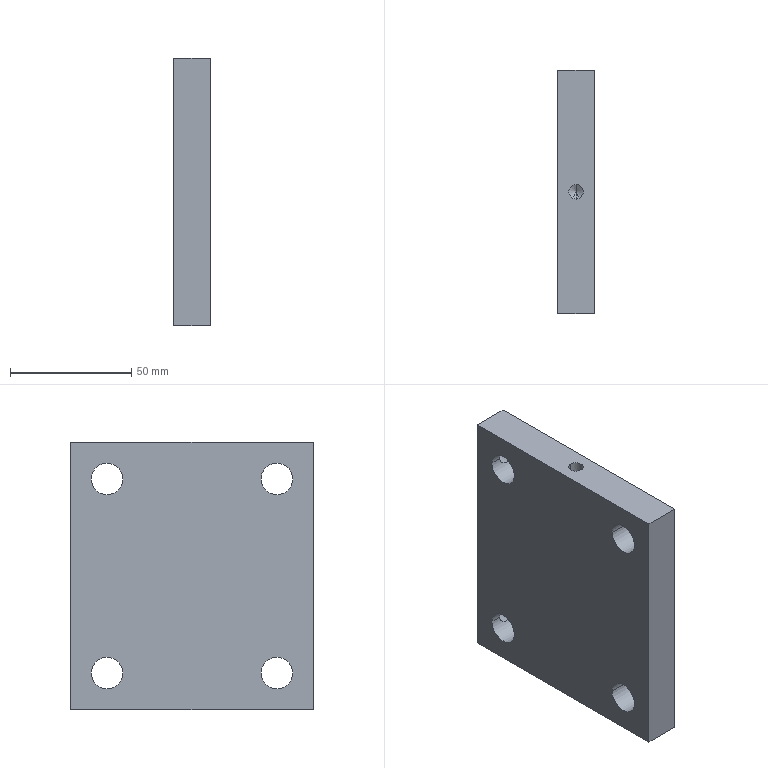Part | STEP file | Positioning_id2118_x_t | 1 solid | 32 faces | box 15 x 100 x 110 mm | volume 155502 mm3 | cylinder 22 | plane 6 | cone 4 | commonest cylinder face diameters 6 x12 13 x8 14 x2